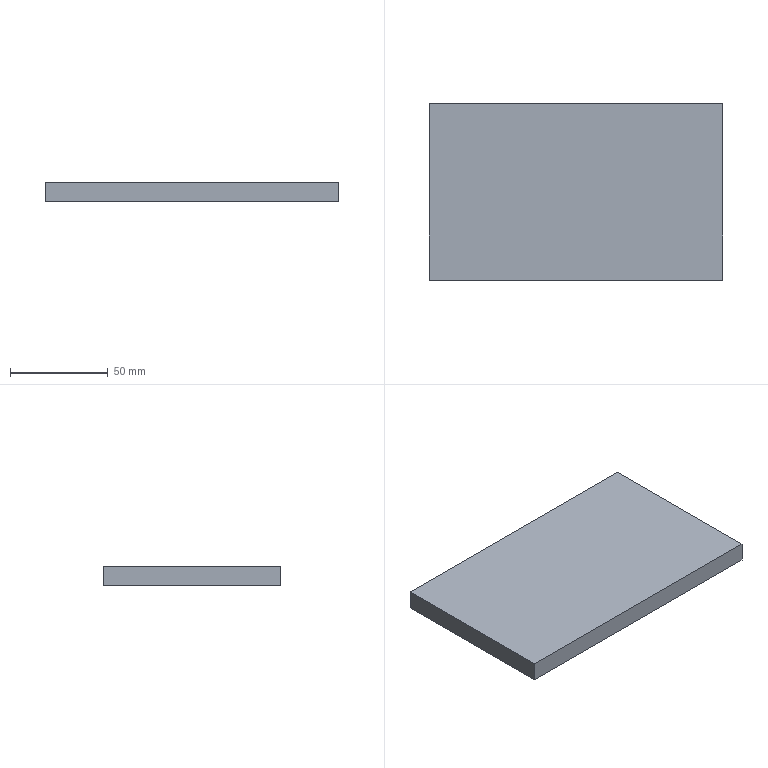Part | SolidWorks | features Extrusion 1 | 1 solid | 6 faces | box 150 x 90 x 10 mm | volume 135000 mm3 | plane 6
STEP:
#1=CARTESIAN_POINT('',(0.,90.,0.));
#2=VERTEX_POINT('',#1);
#3=CARTESIAN_POINT('',(0.,0.,0.));
#4=VERTEX_POINT('',#3);
#5=CARTESIAN_POINT('',(0.,90.,0.));
#6=DIRECTION('',(0.,-1.,0.));
#7=VECTOR('',#6,1000.);
#8=LINE('',#5,#7);
#9=EDGE_CURVE('',#2,#4,#8,.T.);
#10=ORIENTED_EDGE('',*,*,#9,.T.);
#11=CARTESIAN_POINT('',(0.,0.,10.));
#12=VERTEX_POINT('',#11);
#13=CARTESIAN_POINT('',(0.,0.,10.));
#14=DIRECTION('',(0.,0.,-1.));
#15=VECTOR('',#14,1000.);
#16=LINE('',#13,#15);
#17=EDGE_CURVE('',#12,#4,#16,.T.);
#18=ORIENTED_EDGE('',*,*,#17,.F.);
#19=CARTESIAN_POINT('',(0.,90.,10.));
#20=VERTEX_POINT('',#19);
#21=CARTESIAN_POINT('',(0.,90.,10.));
#22=DIRECTION('',(0.,-1.,0.));
#23=VECTOR('',#22,1000.);
#24=LINE('',#21,#23);
#25=EDGE_CURVE('',#20,#12,#24,.T.);
#26=ORIENTED_EDGE('',*,*,#25,.F.);
#27=CARTESIAN_POINT('',(0.,90.,10.));
#28=DIRECTION('',(0.,0.,-1.));
#29=VECTOR('',#28,1000.);
#30=LINE('',#27,#29);
#31=EDGE_CURVE('',#20,#2,#30,.T.);
#32=ORIENTED_EDGE('',*,*,#31,.T.);
#33=EDGE_LOOP('',(#10,#18,#26,#32));
#34=FACE_OUTER_BOUND('',#33,.T.);
#35=CARTESIAN_POINT('',(0.,90.,10.));
#36=DIRECTION('',(1.,0.,0.));
#37=DIRECTION('',(0.,0.,-1.));
#38=AXIS2_PLACEMENT_3D('',#35,#36,#37);
#39=PLANE('',#38);
#40=ADVANCED_FACE('',(#34),#39,.F.);
#41=CARTESIAN_POINT('',(150.,0.,0.));
#42=VERTEX_POINT('',#41);
#43=CARTESIAN_POINT('',(0.,0.,0.));
#44=DIRECTION('',(1.,0.,0.));
#45=VECTOR('',#44,1000.);
#46=LINE('',#43,#45);
#47=EDGE_CURVE('',#4,#42,#46,.T.);
#48=ORIENTED_EDGE('',*,*,#47,.T.);
#49=CARTESIAN_POINT('',(150.,0.,10.));
#50=VERTEX_POINT('',#49);
#51=CARTESIAN_POINT('',(150.,0.,10.));
#52=DIRECTION('',(0.,0.,-1.));
#53=VECTOR('',#52,1000.);
#54=LINE('',#51,#53);
#55=EDGE_CURVE('',#50,#42,#54,.T.);
#56=ORIENTED_EDGE('',*,*,#55,.F.);
#57=CARTESIAN_POINT('',(0.,0.,10.));
#58=DIRECTION('',(1.,0.,0.));
#59=VECTOR('',#58,1000.);
#60=LINE('',#57,#59);
#61=EDGE_CURVE('',#12,#50,#60,.T.);
#62=ORIENTED_EDGE('',*,*,#61,.F.);
#63=ORIENTED_EDGE('',*,*,#17,.T.);
#64=EDGE_LOOP('',(#48,#56,#62,#63));
#65=FACE_OUTER_BOUND('',#64,.T.);
#66=CARTESIAN_POINT('',(0.,0.,10.));
#67=DIRECTION('',(0.,1.,0.));
#68=DIRECTION('',(0.,0.,1.));
#69=AXIS2_PLACEMENT_3D('',#66,#67,#68);
#70=PLANE('',#69);
#71=ADVANCED_FACE('',(#65),#70,.F.);
#72=CARTESIAN_POINT('',(150.,90.,0.));
#73=VERTEX_POINT('',#72);
#74=CARTESIAN_POINT('',(150.,0.,0.));
#75=DIRECTION('',(0.,1.,0.));
#76=VECTOR('',#75,1000.);
#77=LINE('',#74,#76);
#78=EDGE_CURVE('',#42,#73,#77,.T.);
#79=ORIENTED_EDGE('',*,*,#78,.T.);
#80=CARTESIAN_POINT('',(150.,90.,10.));
#81=VERTEX_POINT('',#80);
#82=CARTESIAN_POINT('',(150.,90.,10.));
#83=DIRECTION('',(0.,0.,-1.));
#84=VECTOR('',#83,1000.);
#85=LINE('',#82,#84);
#86=EDGE_CURVE('',#81,#73,#85,.T.);
#87=ORIENTED_EDGE('',*,*,#86,.F.);
#88=CARTESIAN_POINT('',(150.,0.,10.));
#89=DIRECTION('',(0.,1.,0.));
#90=VECTOR('',#89,1000.);
#91=LINE('',#88,#90);
#92=EDGE_CURVE('',#50,#81,#91,.T.);
#93=ORIENTED_EDGE('',*,*,#92,.F.);
#94=ORIENTED_EDGE('',*,*,#55,.T.);
#95=EDGE_LOOP('',(#79,#87,#93,#94));
#96=FACE_OUTER_BOUND('',#95,.T.);
#97=CARTESIAN_POINT('',(150.,0.,10.));
#98=DIRECTION('',(-1.,0.,0.));
#99=DIRECTION('',(0.,0.,1.));
#100=AXIS2_PLACEMENT_3D('',#97,#98,#99);
#101=PLANE('',#100);
#102=ADVANCED_FACE('',(#96),#101,.F.);
#103=CARTESIAN_POINT('',(150.,90.,0.));
#104=DIRECTION('',(-1.,0.,0.));
#105=VECTOR('',#104,1000.);
#106=LINE('',#103,#105);
#107=EDGE_CURVE('',#73,#2,#106,.T.);
#108=ORIENTED_EDGE('',*,*,#107,.T.);
#109=ORIENTED_EDGE('',*,*,#31,.F.);
#110=CARTESIAN_POINT('',(150.,90.,10.));
#111=DIRECTION('',(-1.,0.,0.));
#112=VECTOR('',#111,1000.);
#113=LINE('',#110,#112);
#114=EDGE_CURVE('',#81,#20,#113,.T.);
#115=ORIENTED_EDGE('',*,*,#114,.F.);
#116=ORIENTED_EDGE('',*,*,#86,.T.);
#117=EDGE_LOOP('',(#108,#109,#115,#116));
#118=FACE_OUTER_BOUND('',#117,.T.);
#119=CARTESIAN_POINT('',(150.,90.,10.));
#120=DIRECTION('',(0.,-1.,0.));
#121=DIRECTION('',(0.,0.,-1.));
#122=AXIS2_PLACEMENT_3D('',#119,#120,#121);
#123=PLANE('',#122);
#124=ADVANCED_FACE('',(#118),#123,.F.);
#125=ORIENTED_EDGE('',*,*,#25,.T.);
#126=ORIENTED_EDGE('',*,*,#61,.T.);
#127=ORIENTED_EDGE('',*,*,#92,.T.);
#128=ORIENTED_EDGE('',*,*,#114,.T.);
#129=EDGE_LOOP('',(#125,#126,#127,#128));
#130=FACE_OUTER_BOUND('',#129,.T.);
#131=CARTESIAN_POINT('',(0.,0.,10.));
#132=DIRECTION('',(0.,0.,1.));
#133=DIRECTION('',(1.,0.,0.));
#134=AXIS2_PLACEMENT_3D('',#131,#132,#133);
#135=PLANE('',#134);
#136=ADVANCED_FACE('',(#130),#135,.T.);
#137=ORIENTED_EDGE('',*,*,#9,.F.);
#138=ORIENTED_EDGE('',*,*,#107,.F.);
#139=ORIENTED_EDGE('',*,*,#78,.F.);
#140=ORIENTED_EDGE('',*,*,#47,.F.);
#141=EDGE_LOOP('',(#137,#138,#139,#140));
#142=FACE_OUTER_BOUND('',#141,.T.);
#143=CARTESIAN_POINT('',(0.,0.,0.));
#144=DIRECTION('',(0.,0.,1.));
#145=DIRECTION('',(1.,0.,0.));
#146=AXIS2_PLACEMENT_3D('',#143,#144,#145);
#147=PLANE('',#146);
#148=ADVANCED_FACE('',(#142),#147,.F.);
#149=CLOSED_SHELL('',(#40,#71,#102,#124,#136,#148));
#150=MANIFOLD_SOLID_BREP('',#149);
#151=CARTESIAN_POINT('',(0.,0.,0.));
#152=DIRECTION('',(0.,0.,1.));
#153=DIRECTION('',(1.,0.,0.));
#154=AXIS2_PLACEMENT_3D('',#151,#152,#153);
#155=(LENGTH_UNIT()NAMED_UNIT(*)SI_UNIT(.MILLI.,.METRE.));
#156=UNCERTAINTY_MEASURE_WITH_UNIT(LENGTH_MEASURE(0.00001),#155,'','');
#157=(NAMED_UNIT(*)PLANE_ANGLE_UNIT()SI_UNIT($,.RADIAN.));
#158=(NAMED_UNIT(*)SI_UNIT($,.STERADIAN.)SOLID_ANGLE_UNIT());
#159=(GEOMETRIC_REPRESENTATION_CONTEXT(3)GLOBAL_UNCERTAINTY_ASSIGNED_CONTEXT((#156))GLOBAL_UNIT_ASSIGNED_CONTEXT((#155,#157,#158))REPRESENTATION_CONTEXT('',''));
#160=ADVANCED_BREP_SHAPE_REPRESENTATION('',(#150,#154),#159);